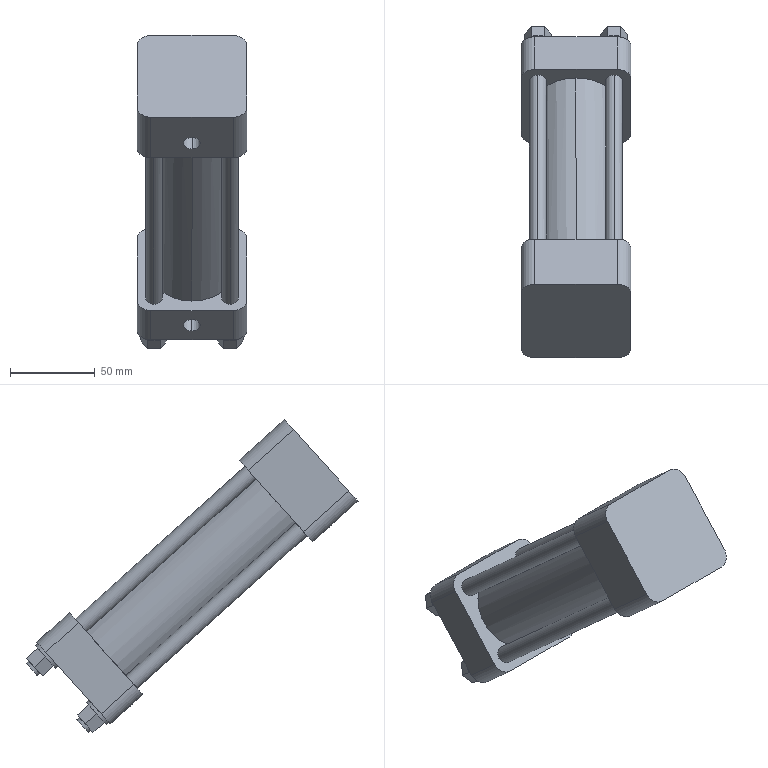Part | Creo | 1 solid | 88 faces | box 65 x 196.293 x 185.154 mm | volume 569697 mm3 | plane 50 | cylinder 38 | commonest cylinder face diameters 10 x20 16 x8 18 x8 50 x2